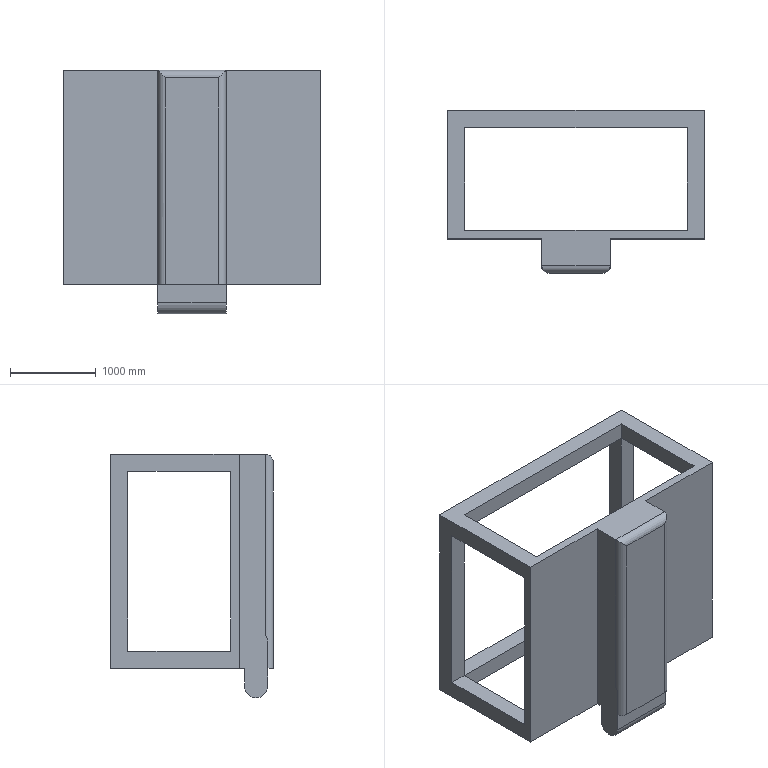Part | SolidWorks | features ICE 6, Extrusion 1, Fillet 1 | 1 solid | 36 faces | box 3000 x 1900 x 2845 mm | volume 2208765977 mm3 | plane 30 | cylinder 6 | commonest cylinder face diameters 180 x3 271.424 x3
STEP:
#1=CARTESIAN_POINT('',(-1300.,300.,10000.));
#2=VERTEX_POINT('',#1);
#3=CARTESIAN_POINT('',(-1300.,1500.,10000.));
#4=VERTEX_POINT('',#3);
#5=CARTESIAN_POINT('',(-1300.,1500.,10000.));
#6=DIRECTION('',(0.,1.,0.));
#7=VECTOR('',#6,1000.);
#8=LINE('',#5,#7);
#9=EDGE_CURVE('',#2,#4,#8,.T.);
#10=ORIENTED_EDGE('',*,*,#9,.F.);
#11=CARTESIAN_POINT('',(1300.,300.,10000.));
#12=VERTEX_POINT('',#11);
#13=CARTESIAN_POINT('',(1300.,300.,10000.));
#14=DIRECTION('',(-1.,0.,0.));
#15=VECTOR('',#14,1000.);
#16=LINE('',#13,#15);
#17=EDGE_CURVE('',#12,#2,#16,.T.);
#18=ORIENTED_EDGE('',*,*,#17,.F.);
#19=CARTESIAN_POINT('',(1300.,1500.,10000.));
#20=VERTEX_POINT('',#19);
#21=CARTESIAN_POINT('',(1300.,1500.,10000.));
#22=DIRECTION('',(0.,-1.,0.));
#23=VECTOR('',#22,1000.);
#24=LINE('',#21,#23);
#25=EDGE_CURVE('',#20,#12,#24,.T.);
#26=ORIENTED_EDGE('',*,*,#25,.F.);
#27=CARTESIAN_POINT('',(1300.,1500.,10000.));
#28=DIRECTION('',(1.,0.,0.));
#29=VECTOR('',#28,1000.);
#30=LINE('',#27,#29);
#31=EDGE_CURVE('',#4,#20,#30,.T.);
#32=ORIENTED_EDGE('',*,*,#31,.F.);
#33=EDGE_LOOP('',(#10,#18,#26,#32));
#34=FACE_BOUND('',#33,.T.);
#35=CARTESIAN_POINT('',(400.,135.712,10000.));
#36=VERTEX_POINT('',#35);
#37=CARTESIAN_POINT('',(400.,200.,10000.));
#38=VERTEX_POINT('',#37);
#39=CARTESIAN_POINT('',(400.,200.,10000.));
#40=DIRECTION('',(0.,1.,0.));
#41=VECTOR('',#40,1000.);
#42=LINE('',#39,#41);
#43=EDGE_CURVE('',#36,#38,#42,.T.);
#44=ORIENTED_EDGE('',*,*,#43,.F.);
#45=CARTESIAN_POINT('',(-400.,135.712,10000.));
#46=VERTEX_POINT('',#45);
#47=CARTESIAN_POINT('',(-1500.,135.712,10000.));
#48=DIRECTION('',(-1.,0.,0.));
#49=VECTOR('',#48,1000.);
#50=LINE('',#47,#49);
#51=EDGE_CURVE('',#36,#46,#50,.T.);
#52=ORIENTED_EDGE('',*,*,#51,.T.);
#53=CARTESIAN_POINT('',(-400.,200.,10000.));
#54=VERTEX_POINT('',#53);
#55=CARTESIAN_POINT('',(-400.,200.,10000.));
#56=DIRECTION('',(0.,-1.,0.));
#57=VECTOR('',#56,1000.);
#58=LINE('',#55,#57);
#59=EDGE_CURVE('',#54,#46,#58,.T.);
#60=ORIENTED_EDGE('',*,*,#59,.F.);
#61=CARTESIAN_POINT('',(-1500.,200.,10000.));
#62=VERTEX_POINT('',#61);
#63=CARTESIAN_POINT('',(-1500.,200.,10000.));
#64=DIRECTION('',(-1.,0.,0.));
#65=VECTOR('',#64,1000.);
#66=LINE('',#63,#65);
#67=EDGE_CURVE('',#54,#62,#66,.T.);
#68=ORIENTED_EDGE('',*,*,#67,.T.);
#69=CARTESIAN_POINT('',(-1500.,1700.,10000.));
#70=VERTEX_POINT('',#69);
#71=CARTESIAN_POINT('',(-1500.,1700.,10000.));
#72=DIRECTION('',(0.,-1.,0.));
#73=VECTOR('',#72,1000.);
#74=LINE('',#71,#73);
#75=EDGE_CURVE('',#70,#62,#74,.T.);
#76=ORIENTED_EDGE('',*,*,#75,.F.);
#77=CARTESIAN_POINT('',(1500.,1700.,10000.));
#78=VERTEX_POINT('',#77);
#79=CARTESIAN_POINT('',(-1500.,1700.,10000.));
#80=DIRECTION('',(-1.,0.,0.));
#81=VECTOR('',#80,1000.);
#82=LINE('',#79,#81);
#83=EDGE_CURVE('',#78,#70,#82,.T.);
#84=ORIENTED_EDGE('',*,*,#83,.F.);
#85=CARTESIAN_POINT('',(1500.,200.,10000.));
#86=VERTEX_POINT('',#85);
#87=CARTESIAN_POINT('',(1500.,1700.,10000.));
#88=DIRECTION('',(0.,-1.,0.));
#89=VECTOR('',#88,1000.);
#90=LINE('',#87,#89);
#91=EDGE_CURVE('',#78,#86,#90,.T.);
#92=ORIENTED_EDGE('',*,*,#91,.T.);
#93=CARTESIAN_POINT('',(-1500.,200.,10000.));
#94=DIRECTION('',(-1.,0.,0.));
#95=VECTOR('',#94,1000.);
#96=LINE('',#93,#95);
#97=EDGE_CURVE('',#86,#38,#96,.T.);
#98=ORIENTED_EDGE('',*,*,#97,.T.);
#99=EDGE_LOOP('',(#44,#52,#60,#68,#76,#84,#92,#98));
#100=FACE_OUTER_BOUND('',#99,.T.);
#101=CARTESIAN_POINT('',(-1500.,1700.,10000.));
#102=DIRECTION('',(0.,0.,1.));
#103=DIRECTION('',(1.,0.,0.));
#104=AXIS2_PLACEMENT_3D('',#101,#102,#103);
#105=PLANE('',#104);
#106=ADVANCED_FACE('',(#34,#100),#105,.F.);
#107=CARTESIAN_POINT('',(400.,-110.,12500.));
#108=VERTEX_POINT('',#107);
#109=CARTESIAN_POINT('',(400.,-110.,10383.617));
#110=VERTEX_POINT('',#109);
#111=CARTESIAN_POINT('',(400.,-110.,12500.));
#112=DIRECTION('',(0.,0.,-1.));
#113=VECTOR('',#112,1000.);
#114=LINE('',#111,#113);
#115=EDGE_CURVE('',#108,#110,#114,.T.);
#116=ORIENTED_EDGE('',*,*,#115,.T.);
#117=CARTESIAN_POINT('',(400.,-135.712,10304.133));
#118=VERTEX_POINT('',#117);
#119=CARTESIAN_POINT('',(400.,0.,10304.133));
#120=DIRECTION('',(1.,0.,0.));
#121=DIRECTION('',(0.,1.,0.));
#122=AXIS2_PLACEMENT_3D('',#119,#120,#121);
#123=CIRCLE('',#122,135.712);
#124=EDGE_CURVE('',#110,#118,#123,.T.);
#125=ORIENTED_EDGE('',*,*,#124,.T.);
#126=CARTESIAN_POINT('',(400.,-135.712,9790.264));
#127=VERTEX_POINT('',#126);
#128=CARTESIAN_POINT('',(400.,-135.712,10304.133));
#129=DIRECTION('',(0.,0.,-1.));
#130=VECTOR('',#129,1000.);
#131=LINE('',#128,#130);
#132=EDGE_CURVE('',#118,#127,#131,.T.);
#133=ORIENTED_EDGE('',*,*,#132,.T.);
#134=CARTESIAN_POINT('',(400.,135.712,9790.264));
#135=VERTEX_POINT('',#134);
#136=CARTESIAN_POINT('',(400.,0.,9790.264));
#137=DIRECTION('',(1.,0.,0.));
#138=DIRECTION('',(0.,1.,0.));
#139=AXIS2_PLACEMENT_3D('',#136,#137,#138);
#140=CIRCLE('',#139,135.712);
#141=EDGE_CURVE('',#127,#135,#140,.T.);
#142=ORIENTED_EDGE('',*,*,#141,.T.);
#143=CARTESIAN_POINT('',(400.,135.712,10304.133));
#144=DIRECTION('',(0.,0.,1.));
#145=VECTOR('',#144,1000.);
#146=LINE('',#143,#145);
#147=EDGE_CURVE('',#135,#36,#146,.T.);
#148=ORIENTED_EDGE('',*,*,#147,.T.);
#149=ORIENTED_EDGE('',*,*,#43,.T.);
#150=CARTESIAN_POINT('',(400.,200.,12500.));
#151=VERTEX_POINT('',#150);
#152=CARTESIAN_POINT('',(400.,200.,12500.));
#153=DIRECTION('',(0.,0.,-1.));
#154=VECTOR('',#153,1000.);
#155=LINE('',#152,#154);
#156=EDGE_CURVE('',#151,#38,#155,.T.);
#157=ORIENTED_EDGE('',*,*,#156,.F.);
#158=CARTESIAN_POINT('',(400.,200.,12500.));
#159=DIRECTION('',(0.,1.,0.));
#160=VECTOR('',#159,1000.);
#161=LINE('',#158,#160);
#162=EDGE_CURVE('',#108,#151,#161,.T.);
#163=ORIENTED_EDGE('',*,*,#162,.F.);
#164=EDGE_LOOP('',(#116,#125,#133,#142,#148,#149,#157,#163));
#165=FACE_OUTER_BOUND('',#164,.T.);
#166=CARTESIAN_POINT('',(400.,200.,12500.));
#167=DIRECTION('',(-1.,0.,0.));
#168=DIRECTION('',(0.,-1.,0.));
#169=AXIS2_PLACEMENT_3D('',#166,#167,#168);
#170=PLANE('',#169);
#171=ADVANCED_FACE('',(#165),#170,.F.);
#172=CARTESIAN_POINT('',(-400.,-135.712,10304.133));
#173=VERTEX_POINT('',#172);
#174=CARTESIAN_POINT('',(-400.,-110.,10383.617));
#175=VERTEX_POINT('',#174);
#176=CARTESIAN_POINT('',(-400.,0.,10304.133));
#177=DIRECTION('',(-1.,0.,0.));
#178=DIRECTION('',(0.,1.,0.));
#179=AXIS2_PLACEMENT_3D('',#176,#177,#178);
#180=CIRCLE('',#179,135.712);
#181=EDGE_CURVE('',#173,#175,#180,.T.);
#182=ORIENTED_EDGE('',*,*,#181,.T.);
#183=CARTESIAN_POINT('',(-400.,-110.,12500.));
#184=VERTEX_POINT('',#183);
#185=CARTESIAN_POINT('',(-400.,-110.,12500.));
#186=DIRECTION('',(0.,0.,1.));
#187=VECTOR('',#186,1000.);
#188=LINE('',#185,#187);
#189=EDGE_CURVE('',#175,#184,#188,.T.);
#190=ORIENTED_EDGE('',*,*,#189,.T.);
#191=CARTESIAN_POINT('',(-400.,200.,12500.));
#192=VERTEX_POINT('',#191);
#193=CARTESIAN_POINT('',(-400.,200.,12500.));
#194=DIRECTION('',(0.,-1.,0.));
#195=VECTOR('',#194,1000.);
#196=LINE('',#193,#195);
#197=EDGE_CURVE('',#192,#184,#196,.T.);
#198=ORIENTED_EDGE('',*,*,#197,.F.);
#199=CARTESIAN_POINT('',(-400.,200.,12500.));
#200=DIRECTION('',(0.,0.,-1.));
#201=VECTOR('',#200,1000.);
#202=LINE('',#199,#201);
#203=EDGE_CURVE('',#192,#54,#202,.T.);
#204=ORIENTED_EDGE('',*,*,#203,.T.);
#205=ORIENTED_EDGE('',*,*,#59,.T.);
#206=CARTESIAN_POINT('',(-400.,135.712,9790.264));
#207=VERTEX_POINT('',#206);
#208=CARTESIAN_POINT('',(-400.,135.712,10304.133));
#209=DIRECTION('',(0.,0.,-1.));
#210=VECTOR('',#209,1000.);
#211=LINE('',#208,#210);
#212=EDGE_CURVE('',#46,#207,#211,.T.);
#213=ORIENTED_EDGE('',*,*,#212,.T.);
#214=CARTESIAN_POINT('',(-400.,-135.712,9790.264));
#215=VERTEX_POINT('',#214);
#216=CARTESIAN_POINT('',(-400.,0.,9790.264));
#217=DIRECTION('',(-1.,0.,0.));
#218=DIRECTION('',(0.,1.,0.));
#219=AXIS2_PLACEMENT_3D('',#216,#217,#218);
#220=CIRCLE('',#219,135.712);
#221=EDGE_CURVE('',#207,#215,#220,.T.);
#222=ORIENTED_EDGE('',*,*,#221,.T.);
#223=CARTESIAN_POINT('',(-400.,-135.712,10304.133));
#224=DIRECTION('',(0.,0.,1.));
#225=VECTOR('',#224,1000.);
#226=LINE('',#223,#225);
#227=EDGE_CURVE('',#215,#173,#226,.T.);
#228=ORIENTED_EDGE('',*,*,#227,.T.);
#229=EDGE_LOOP('',(#182,#190,#198,#204,#205,#213,#222,#228));
#230=FACE_OUTER_BOUND('',#229,.T.);
#231=CARTESIAN_POINT('',(-400.,200.,12500.));
#232=DIRECTION('',(1.,0.,0.));
#233=DIRECTION('',(0.,1.,0.));
#234=AXIS2_PLACEMENT_3D('',#231,#232,#233);
#235=PLANE('',#234);
#236=ADVANCED_FACE('',(#230),#235,.F.);
#237=CARTESIAN_POINT('',(310.,-200.,10000.));
#238=VERTEX_POINT('',#237);
#239=CARTESIAN_POINT('',(-310.,-200.,10000.));
#240=VERTEX_POINT('',#239);
#241=CARTESIAN_POINT('',(-400.,-200.,10000.));
#242=DIRECTION('',(-1.,0.,0.));
#243=VECTOR('',#242,1000.);
#244=LINE('',#241,#243);
#245=EDGE_CURVE('',#238,#240,#244,.T.);
#246=ORIENTED_EDGE('',*,*,#245,.F.);
#247=CARTESIAN_POINT('',(310.,-200.,12410.));
#248=VERTEX_POINT('',#247);
#249=CARTESIAN_POINT('',(310.,-200.,12500.));
#250=DIRECTION('',(0.,0.,1.));
#251=VECTOR('',#250,1000.);
#252=LINE('',#249,#251);
#253=EDGE_CURVE('',#238,#248,#252,.T.);
#254=ORIENTED_EDGE('',*,*,#253,.T.);
#255=CARTESIAN_POINT('',(-310.,-200.,12410.));
#256=VERTEX_POINT('',#255);
#257=CARTESIAN_POINT('',(-400.,-200.,12410.));
#258=DIRECTION('',(-1.,0.,0.));
#259=VECTOR('',#258,1000.);
#260=LINE('',#257,#259);
#261=EDGE_CURVE('',#248,#256,#260,.T.);
#262=ORIENTED_EDGE('',*,*,#261,.T.);
#263=CARTESIAN_POINT('',(-310.,-200.,12500.));
#264=DIRECTION('',(0.,0.,-1.));
#265=VECTOR('',#264,1000.);
#266=LINE('',#263,#265);
#267=EDGE_CURVE('',#256,#240,#266,.T.);
#268=ORIENTED_EDGE('',*,*,#267,.T.);
#269=EDGE_LOOP('',(#246,#254,#262,#268));
#270=FACE_OUTER_BOUND('',#269,.T.);
#271=CARTESIAN_POINT('',(-400.,-200.,12500.));
#272=DIRECTION('',(0.,1.,0.));
#273=DIRECTION('',(0.,0.,1.));
#274=AXIS2_PLACEMENT_3D('',#271,#272,#273);
#275=PLANE('',#274);
#276=ADVANCED_FACE('',(#270),#275,.F.);
#277=CARTESIAN_POINT('',(396.249,-135.712,10304.133));
#278=VERTEX_POINT('',#277);
#279=CARTESIAN_POINT('',(400.,-110.,10383.617));
#280=CARTESIAN_POINT('',(400.,-112.098,10380.714));
#281=CARTESIAN_POINT('',(399.927,-114.065,10377.751));
#282=CARTESIAN_POINT('',(399.685,-117.747,10371.705));
#283=CARTESIAN_POINT('',(399.516,-119.462,10368.624));
#284=CARTESIAN_POINT('',(398.925,-124.237,10359.201));
#285=CARTESIAN_POINT('',(398.422,-126.93,10352.684));
#286=CARTESIAN_POINT('',(397.827,-129.666,10344.227));
#287=CARTESIAN_POINT('',(397.709,-130.183,10342.516));
#288=CARTESIAN_POINT('',(397.482,-131.146,10339.087));
#289=CARTESIAN_POINT('',(397.373,-131.592,10337.368));
#290=CARTESIAN_POINT('',(397.061,-132.826,10332.196));
#291=CARTESIAN_POINT('',(396.877,-133.511,10328.731));
#292=CARTESIAN_POINT('',(396.572,-134.608,10321.765));
#293=CARTESIAN_POINT('',(396.453,-135.021,10318.264));
#294=CARTESIAN_POINT('',(396.291,-135.573,10311.226));
#295=CARTESIAN_POINT('',(396.249,-135.712,10307.689));
#296=CARTESIAN_POINT('',(396.249,-135.712,10304.133));
#297=B_SPLINE_CURVE_WITH_KNOTS('',3,(#279,#280,#281,#282,#283,#284,#285,#286,#287,#288,#289,#290,#291,#292,#293,#294,#295,#296),.UNSPECIFIED.,.F.,.F.,(4,2,2,2,2,2,2,2,4),(0.,0.01058,0.02116,0.04232,0.04761,0.0529,0.06347,0.07405,0.08463),.UNSPECIFIED.);
#298=EDGE_CURVE('',#110,#278,#297,.T.);
#299=ORIENTED_EDGE('',*,*,#298,.F.);
#300=ORIENTED_EDGE('',*,*,#115,.F.);
#301=CARTESIAN_POINT('',(310.,-200.,12410.));
#302=CARTESIAN_POINT('',(362.721,-200.,12462.721));
#303=CARTESIAN_POINT('',(400.,-162.721,12500.));
#304=CARTESIAN_POINT('',(400.,-110.,12500.));
#305=(BOUNDED_CURVE()B_SPLINE_CURVE(3,(#301,#302,#303,#304),.UNSPECIFIED.,.F.,.F.)B_SPLINE_CURVE_WITH_KNOTS((4,4),(1.571,3.142),.UNSPECIFIED.)CURVE()GEOMETRIC_REPRESENTATION_ITEM()RATIONAL_B_SPLINE_CURVE((1.,0.8047,0.8047,1.))REPRESENTATION_ITEM(''));
#306=EDGE_CURVE('',#248,#108,#305,.T.);
#307=ORIENTED_EDGE('',*,*,#306,.F.);
#308=ORIENTED_EDGE('',*,*,#253,.F.);
#309=CARTESIAN_POINT('',(396.249,-135.712,10000.));
#310=VERTEX_POINT('',#309);
#311=CARTESIAN_POINT('',(310.,-110.,10000.));
#312=DIRECTION('',(0.,0.,1.));
#313=DIRECTION('',(-1.,0.,0.));
#314=AXIS2_PLACEMENT_3D('',#311,#312,#313);
#315=CIRCLE('',#314,90.);
#316=EDGE_CURVE('',#238,#310,#315,.T.);
#317=ORIENTED_EDGE('',*,*,#316,.T.);
#318=CARTESIAN_POINT('',(396.249,-135.712,12500.));
#319=DIRECTION('',(0.,0.,-1.));
#320=VECTOR('',#319,1000.);
#321=LINE('',#318,#320);
#322=EDGE_CURVE('',#278,#310,#321,.T.);
#323=ORIENTED_EDGE('',*,*,#322,.F.);
#324=EDGE_LOOP('',(#299,#300,#307,#308,#317,#323));
#325=FACE_OUTER_BOUND('',#324,.T.);
#326=CARTESIAN_POINT('',(310.,-110.,12500.));
#327=DIRECTION('',(0.,0.,-1.));
#328=DIRECTION('',(-1.,0.,0.));
#329=AXIS2_PLACEMENT_3D('',#326,#327,#328);
#330=CYLINDRICAL_SURFACE('',#329,90.);
#331=ADVANCED_FACE('',(#325),#330,.T.);
#332=CARTESIAN_POINT('',(-396.249,-135.712,10304.133));
#333=VERTEX_POINT('',#332);
#334=CARTESIAN_POINT('',(-396.249,-135.712,10304.133));
#335=CARTESIAN_POINT('',(-396.249,-135.712,10305.906));
#336=CARTESIAN_POINT('',(-396.259,-135.677,10307.684));
#337=CARTESIAN_POINT('',(-396.301,-135.537,10311.249));
#338=CARTESIAN_POINT('',(-396.332,-135.432,10313.027));
#339=CARTESIAN_POINT('',(-396.455,-135.014,10318.334));
#340=CARTESIAN_POINT('',(-396.575,-134.598,10321.841));
#341=CARTESIAN_POINT('',(-397.032,-132.949,10332.274));
#342=CARTESIAN_POINT('',(-397.467,-131.317,10339.111));
#343=CARTESIAN_POINT('',(-398.058,-128.604,10347.514));
#344=CARTESIAN_POINT('',(-398.178,-128.027,10349.187));
#345=CARTESIAN_POINT('',(-398.419,-126.806,10352.519));
#346=CARTESIAN_POINT('',(-398.54,-126.159,10354.18));
#347=CARTESIAN_POINT('',(-398.894,-124.13,10359.106));
#348=CARTESIAN_POINT('',(-399.12,-122.654,10362.324));
#349=CARTESIAN_POINT('',(-399.516,-119.459,10368.629));
#350=CARTESIAN_POINT('',(-399.686,-117.74,10371.717));
#351=CARTESIAN_POINT('',(-399.928,-114.056,10377.764));
#352=CARTESIAN_POINT('',(-400.,-112.091,10380.723));
#353=CARTESIAN_POINT('',(-400.,-110.,10383.617));
#354=B_SPLINE_CURVE_WITH_KNOTS('',3,(#334,#335,#336,#337,#338,#339,#340,#341,#342,#343,#344,#345,#346,#347,#348,#349,#350,#351,#352,#353),.UNSPECIFIED.,.F.,.F.,(4,2,2,2,2,2,2,2,2,4),(0.08463,0.08991,0.09518,0.1057,0.1268,0.1321,0.1374,0.1479,0.1585,0.169),.UNSPECIFIED.);
#355=EDGE_CURVE('',#333,#175,#354,.T.);
#356=ORIENTED_EDGE('',*,*,#355,.F.);
#357=CARTESIAN_POINT('',(-396.249,-135.712,10000.));
#358=VERTEX_POINT('',#357);
#359=CARTESIAN_POINT('',(-396.249,-135.712,12500.));
#360=DIRECTION('',(0.,0.,1.));
#361=VECTOR('',#360,1000.);
#362=LINE('',#359,#361);
#363=EDGE_CURVE('',#358,#333,#362,.T.);
#364=ORIENTED_EDGE('',*,*,#363,.F.);
#365=CARTESIAN_POINT('',(-310.,-110.,10000.));
#366=DIRECTION('',(0.,0.,1.));
#367=DIRECTION('',(-1.,0.,0.));
#368=AXIS2_PLACEMENT_3D('',#365,#366,#367);
#369=CIRCLE('',#368,90.);
#370=EDGE_CURVE('',#358,#240,#369,.T.);
#371=ORIENTED_EDGE('',*,*,#370,.T.);
#372=ORIENTED_EDGE('',*,*,#267,.F.);
#373=CARTESIAN_POINT('',(-310.,-200.,12410.));
#374=CARTESIAN_POINT('',(-362.721,-200.,12462.721));
#375=CARTESIAN_POINT('',(-400.,-162.721,12500.));
#376=CARTESIAN_POINT('',(-400.,-110.,12500.));
#377=(BOUNDED_CURVE()B_SPLINE_CURVE(3,(#373,#374,#375,#376),.UNSPECIFIED.,.F.,.F.)B_SPLINE_CURVE_WITH_KNOTS((4,4),(4.712,6.283),.UNSPECIFIED.)CURVE()GEOMETRIC_REPRESENTATION_ITEM()RATIONAL_B_SPLINE_CURVE((1.,0.8047,0.8047,1.))REPRESENTATION_ITEM(''));
#378=EDGE_CURVE('',#256,#184,#377,.T.);
#379=ORIENTED_EDGE('',*,*,#378,.T.);
#380=ORIENTED_EDGE('',*,*,#189,.F.);
#381=EDGE_LOOP('',(#356,#364,#371,#372,#379,#380));
#382=FACE_OUTER_BOUND('',#381,.T.);
#383=CARTESIAN_POINT('',(-310.,-110.,12500.));
#384=DIRECTION('',(0.,0.,-1.));
#385=DIRECTION('',(-1.,0.,0.));
#386=AXIS2_PLACEMENT_3D('',#383,#384,#385);
#387=CYLINDRICAL_SURFACE('',#386,90.);
#388=ADVANCED_FACE('',(#382),#387,.T.);
#389=CARTESIAN_POINT('',(-1500.,1500.,10200.));
#390=VERTEX_POINT('',#389);
#391=CARTESIAN_POINT('',(-1300.,1500.,10200.));
#392=VERTEX_POINT('',#391);
#393=CARTESIAN_POINT('',(-1500.,1500.,10200.));
#394=DIRECTION('',(1.,0.,0.));
#395=VECTOR('',#394,1000.);
#396=LINE('',#393,#395);
#397=EDGE_CURVE('',#390,#392,#396,.T.);
#398=ORIENTED_EDGE('',*,*,#397,.T.);
#399=CARTESIAN_POINT('',(-1300.,1500.,12300.));
#400=VERTEX_POINT('',#399);
#401=CARTESIAN_POINT('',(-1300.,1500.,12300.));
#402=DIRECTION('',(0.,0.,1.));
#403=VECTOR('',#402,1000.);
#404=LINE('',#401,#403);
#405=EDGE_CURVE('',#392,#400,#404,.T.);
#406=ORIENTED_EDGE('',*,*,#405,.T.);
#407=CARTESIAN_POINT('',(-1500.,1500.,12300.));
#408=VERTEX_POINT('',#407);
#409=CARTESIAN_POINT('',(-1500.,1500.,12300.));
#410=DIRECTION('',(1.,0.,0.));
#411=VECTOR('',#410,1000.);
#412=LINE('',#409,#411);
#413=EDGE_CURVE('',#408,#400,#412,.T.);
#414=ORIENTED_EDGE('',*,*,#413,.F.);
#415=CARTESIAN_POINT('',(-1500.,1500.,12300.));
#416=DIRECTION('',(0.,0.,1.));
#417=VECTOR('',#416,1000.);
#418=LINE('',#415,#417);
#419=EDGE_CURVE('',#390,#408,#418,.T.);
#420=ORIENTED_EDGE('',*,*,#419,.F.);
#421=EDGE_LOOP('',(#398,#406,#414,#420));
#422=FACE_OUTER_BOUND('',#421,.T.);
#423=CARTESIAN_POINT('',(-1500.,1500.,12300.));
#424=DIRECTION('',(0.,1.,0.));
#425=DIRECTION('',(0.,0.,1.));
#426=AXIS2_PLACEMENT_3D('',#423,#424,#425);
#427=PLANE('',#426);
#428=ADVANCED_FACE('',(#422),#427,.F.);
#429=CARTESIAN_POINT('',(1300.,1500.,10200.));
#430=VERTEX_POINT('',#429);
#431=CARTESIAN_POINT('',(1300.,1500.,13000.));
#432=DIRECTION('',(0.,0.,-1.));
#433=VECTOR('',#432,1000.);
#434=LINE('',#431,#433);
#435=EDGE_CURVE('',#430,#20,#434,.T.);
#436=ORIENTED_EDGE('',*,*,#435,.F.);
#437=CARTESIAN_POINT('',(-1500.,1500.,10200.));
#438=DIRECTION('',(-1.,0.,0.));
#439=VECTOR('',#438,1000.);
#440=LINE('',#437,#439);
#441=EDGE_CURVE('',#430,#392,#440,.T.);
#442=ORIENTED_EDGE('',*,*,#441,.T.);
#443=CARTESIAN_POINT('',(-1300.,1500.,13000.));
#444=DIRECTION('',(0.,0.,-1.));
#445=VECTOR('',#444,1000.);
#446=LINE('',#443,#445);
#447=EDGE_CURVE('',#392,#4,#446,.T.);
#448=ORIENTED_EDGE('',*,*,#447,.T.);
#449=ORIENTED_EDGE('',*,*,#31,.T.);
#450=EDGE_LOOP('',(#436,#442,#448,#449));
#451=FACE_OUTER_BOUND('',#450,.T.);
#452=CARTESIAN_POINT('',(-1500.,1500.,12300.));
#453=DIRECTION('',(0.,1.,0.));
#454=DIRECTION('',(0.,0.,1.));
#455=AXIS2_PLACEMENT_3D('',#452,#453,#454);
#456=PLANE('',#455);
#457=ADVANCED_FACE('',(#451),#456,.F.);
#458=CARTESIAN_POINT('',(1300.,1500.,12300.));
#459=VERTEX_POINT('',#458);
#460=CARTESIAN_POINT('',(1500.,1500.,12300.));
#461=VERTEX_POINT('',#460);
#462=CARTESIAN_POINT('',(-1500.,1500.,12300.));
#463=DIRECTION('',(1.,0.,0.));
#464=VECTOR('',#463,1000.);
#465=LINE('',#462,#464);
#466=EDGE_CURVE('',#459,#461,#465,.T.);
#467=ORIENTED_EDGE('',*,*,#466,.F.);
#468=CARTESIAN_POINT('',(1300.,1500.,12300.));
#469=DIRECTION('',(0.,0.,-1.));
#470=VECTOR('',#469,1000.);
#471=LINE('',#468,#470);
#472=EDGE_CURVE('',#459,#430,#471,.T.);
#473=ORIENTED_EDGE('',*,*,#472,.T.);
#474=CARTESIAN_POINT('',(1500.,1500.,10200.));
#475=VERTEX_POINT('',#474);
#476=CARTESIAN_POINT('',(-1500.,1500.,10200.));
#477=DIRECTION('',(1.,0.,0.));
#478=VECTOR('',#477,1000.);
#479=LINE('',#476,#478);
#480=EDGE_CURVE('',#430,#475,#479,.T.);
#481=ORIENTED_EDGE('',*,*,#480,.T.);
#482=CARTESIAN_POINT('',(1500.,1500.,12300.));
#483=DIRECTION('',(0.,0.,1.));
#484=VECTOR('',#483,1000.);
#485=LINE('',#482,#484);
#486=EDGE_CURVE('',#475,#461,#485,.T.);
#487=ORIENTED_EDGE('',*,*,#486,.T.);
#488=EDGE_LOOP('',(#467,#473,#481,#487));
#489=FACE_OUTER_BOUND('',#488,.T.);
#490=CARTESIAN_POINT('',(-1500.,1500.,12300.));
#491=DIRECTION('',(0.,1.,0.));
#492=DIRECTION('',(0.,0.,1.));
#493=AXIS2_PLACEMENT_3D('',#490,#491,#492);
#494=PLANE('',#493);
#495=ADVANCED_FACE('',(#489),#494,.F.);
#496=CARTESIAN_POINT('',(1300.,300.,12300.));
#497=VERTEX_POINT('',#496);
#498=CARTESIAN_POINT('',(1500.,300.,12300.));
#499=VERTEX_POINT('',#498);
#500=CARTESIAN_POINT('',(-1500.,300.,12300.));
#501=DIRECTION('',(1.,0.,0.));
#502=VECTOR('',#501,1000.);
#503=LINE('',#500,#502);
#504=EDGE_CURVE('',#497,#499,#503,.T.);
#505=ORIENTED_EDGE('',*,*,#504,.F.);
#506=CARTESIAN_POINT('',(1300.,1500.,12300.));
#507=DIRECTION('',(0.,1.,0.));
#508=VECTOR('',#507,1000.);
#509=LINE('',#506,#508);
#510=EDGE_CURVE('',#497,#459,#509,.T.);
#511=ORIENTED_EDGE('',*,*,#510,.T.);
#512=ORIENTED_EDGE('',*,*,#466,.T.);
#513=CARTESIAN_POINT('',(1500.,1500.,12300.));
#514=DIRECTION('',(0.,-1.,0.));
#515=VECTOR('',#514,1000.);
#516=LINE('',#513,#515);
#517=EDGE_CURVE('',#461,#499,#516,.T.);
#518=ORIENTED_EDGE('',*,*,#517,.T.);
#519=EDGE_LOOP('',(#505,#511,#512,#518));
#520=FACE_OUTER_BOUND('',#519,.T.);
#521=CARTESIAN_POINT('',(-1500.,1500.,12300.));
#522=DIRECTION('',(0.,0.,1.));
#523=DIRECTION('',(1.,0.,0.));
#524=AXIS2_PLACEMENT_3D('',#521,#522,#523);
#525=PLANE('',#524);
#526=ADVANCED_FACE('',(#520),#525,.F.);
#527=ORIENTED_EDGE('',*,*,#480,.F.);
#528=CARTESIAN_POINT('',(1300.,300.,10200.));
#529=VERTEX_POINT('',#528);
#530=CARTESIAN_POINT('',(1300.,1500.,10200.));
#531=DIRECTION('',(0.,-1.,0.));
#532=VECTOR('',#531,1000.);
#533=LINE('',#530,#532);
#534=EDGE_CURVE('',#430,#529,#533,.T.);
#535=ORIENTED_EDGE('',*,*,#534,.T.);
#536=CARTESIAN_POINT('',(1500.,300.,10200.));
#537=VERTEX_POINT('',#536);
#538=CARTESIAN_POINT('',(-1500.,300.,10200.));
#539=DIRECTION('',(1.,0.,0.));
#540=VECTOR('',#539,1000.);
#541=LINE('',#538,#540);
#542=EDGE_CURVE('',#529,#537,#541,.T.);
#543=ORIENTED_EDGE('',*,*,#542,.T.);
#544=CARTESIAN_POINT('',(1500.,1500.,10200.));
#545=DIRECTION('',(0.,1.,0.));
#546=VECTOR('',#545,1000.);
#547=LINE('',#544,#546);
#548=EDGE_CURVE('',#537,#475,#547,.T.);
#549=ORIENTED_EDGE('',*,*,#548,.T.);
#550=EDGE_LOOP('',(#527,#535,#543,#549));
#551=FACE_OUTER_BOUND('',#550,.T.);
#552=CARTESIAN_POINT('',(-1500.,1500.,10200.));
#553=DIRECTION('',(0.,0.,-1.));
#554=DIRECTION('',(-1.,0.,0.));
#555=AXIS2_PLACEMENT_3D('',#552,#553,#554);
#556=PLANE('',#555);
#557=ADVANCED_FACE('',(#551),#556,.F.);
#558=CARTESIAN_POINT('',(1300.,300.,12500.));
#559=VERTEX_POINT('',#558);
#560=CARTESIAN_POINT('',(1300.,1500.,12500.));
#561=VERTEX_POINT('',#560);
#562=CARTESIAN_POINT('',(1300.,0.,12500.));
#563=DIRECTION('',(0.,1.,0.));
#564=VECTOR('',#563,1000.);
#565=LINE('',#562,#564);
#566=EDGE_CURVE('',#559,#561,#565,.T.);
#567=ORIENTED_EDGE('',*,*,#566,.F.);
#568=CARTESIAN_POINT('',(-1300.,300.,12500.));
#569=VERTEX_POINT('',#568);
#570=CARTESIAN_POINT('',(0.,300.,12500.));
#571=DIRECTION('',(1.,0.,0.));
#572=VECTOR('',#571,1000.);
#573=LINE('',#570,#572);
#574=EDGE_CURVE('',#569,#559,#573,.T.);
#575=ORIENTED_EDGE('',*,*,#574,.F.);
#576=CARTESIAN_POINT('',(-1300.,1500.,12500.));
#577=VERTEX_POINT('',#576);
#578=CARTESIAN_POINT('',(-1300.,0.,12500.));
#579=DIRECTION('',(0.,-1.,0.));
#580=VECTOR('',#579,1000.);
#581=LINE('',#578,#580);
#582=EDGE_CURVE('',#577,#569,#581,.T.);
#583=ORIENTED_EDGE('',*,*,#582,.F.);
#584=CARTESIAN_POINT('',(0.,1500.,12500.));
#585=DIRECTION('',(-1.,0.,0.));
#586=VECTOR('',#585,1000.);
#587=LINE('',#584,#586);
#588=EDGE_CURVE('',#561,#577,#587,.T.);
#589=ORIENTED_EDGE('',*,*,#588,.F.);
#590=EDGE_LOOP('',(#567,#575,#583,#589));
#591=FACE_BOUND('',#590,.T.);
#592=ORIENTED_EDGE('',*,*,#197,.T.);
#593=CARTESIAN_POINT('',(400.,-110.,12500.));
#594=DIRECTION('',(1.,0.,0.));
#595=VECTOR('',#594,1000.);
#596=LINE('',#593,#595);
#597=EDGE_CURVE('',#184,#108,#596,.T.);
#598=ORIENTED_EDGE('',*,*,#597,.T.);
#599=ORIENTED_EDGE('',*,*,#162,.T.);
#600=CARTESIAN_POINT('',(1500.,200.,12500.));
#601=VERTEX_POINT('',#600);
#602=CARTESIAN_POINT('',(-1500.,200.,12500.));
#603=DIRECTION('',(1.,0.,0.));
#604=VECTOR('',#603,1000.);
#605=LINE('',#602,#604);
#606=EDGE_CURVE('',#151,#601,#605,.T.);
#607=ORIENTED_EDGE('',*,*,#606,.T.);
#608=CARTESIAN_POINT('',(1500.,1700.,12500.));
#609=VERTEX_POINT('',#608);
#610=CARTESIAN_POINT('',(1500.,1700.,12500.));
#611=DIRECTION('',(0.,-1.,0.));
#612=VECTOR('',#611,1000.);
#613=LINE('',#610,#612);
#614=EDGE_CURVE('',#609,#601,#613,.T.);
#615=ORIENTED_EDGE('',*,*,#614,.F.);
#616=CARTESIAN_POINT('',(-1500.,1700.,12500.));
#617=VERTEX_POINT('',#616);
#618=CARTESIAN_POINT('',(-1500.,1700.,12500.));
#619=DIRECTION('',(1.,0.,0.));
#620=VECTOR('',#619,1000.);
#621=LINE('',#618,#620);
#622=EDGE_CURVE('',#617,#609,#621,.T.);
#623=ORIENTED_EDGE('',*,*,#622,.F.);
#624=CARTESIAN_POINT('',(-1500.,200.,12500.));
#625=VERTEX_POINT('',#624);
#626=CARTESIAN_POINT('',(-1500.,1700.,12500.));
#627=DIRECTION('',(0.,-1.,0.));
#628=VECTOR('',#627,1000.);
#629=LINE('',#626,#628);
#630=EDGE_CURVE('',#617,#625,#629,.T.);
#631=ORIENTED_EDGE('',*,*,#630,.T.);
#632=CARTESIAN_POINT('',(-1500.,200.,12500.));
#633=DIRECTION('',(1.,0.,0.));
#634=VECTOR('',#633,1000.);
#635=LINE('',#632,#634);
#636=EDGE_CURVE('',#625,#192,#635,.T.);
#637=ORIENTED_EDGE('',*,*,#636,.T.);
#638=EDGE_LOOP('',(#592,#598,#599,#607,#615,#623,#631,#637));
#639=FACE_OUTER_BOUND('',#638,.T.);
#640=CARTESIAN_POINT('',(0.,0.,12500.));
#641=DIRECTION('',(0.,0.,1.));
#642=DIRECTION('',(1.,0.,0.));
#643=AXIS2_PLACEMENT_3D('',#640,#641,#642);
#644=PLANE('',#643);
#645=ADVANCED_FACE('',(#591,#639),#644,.T.);
#646=ORIENTED_EDGE('',*,*,#606,.F.);
#647=ORIENTED_EDGE('',*,*,#156,.T.);
#648=ORIENTED_EDGE('',*,*,#97,.F.);
#649=CARTESIAN_POINT('',(1500.,200.,10000.));
#650=DIRECTION('',(0.,0.,-1.));
#651=VECTOR('',#650,1000.);
#652=LINE('',#649,#651);
#653=EDGE_CURVE('',#601,#86,#652,.T.);
#654=ORIENTED_EDGE('',*,*,#653,.F.);
#655=EDGE_LOOP('',(#646,#647,#648,#654));
#656=FACE_OUTER_BOUND('',#655,.T.);
#657=CARTESIAN_POINT('',(0.,200.,0.));
#658=DIRECTION('',(0.,1.,0.));
#659=DIRECTION('',(0.,0.,1.));
#660=AXIS2_PLACEMENT_3D('',#657,#658,#659);
#661=PLANE('',#660);
#662=ADVANCED_FACE('',(#656),#661,.F.);
#663=CARTESIAN_POINT('',(1500.,300.,12300.));
#664=DIRECTION('',(0.,0.,-1.));
#665=VECTOR('',#664,1000.);
#666=LINE('',#663,#665);
#667=EDGE_CURVE('',#499,#537,#666,.T.);
#668=ORIENTED_EDGE('',*,*,#667,.F.);
#669=ORIENTED_EDGE('',*,*,#517,.F.);
#670=ORIENTED_EDGE('',*,*,#486,.F.);
#671=ORIENTED_EDGE('',*,*,#548,.F.);
#672=EDGE_LOOP('',(#668,#669,#670,#671));
#673=FACE_BOUND('',#672,.T.);
#674=ORIENTED_EDGE('',*,*,#653,.T.);
#675=ORIENTED_EDGE('',*,*,#91,.F.);
#676=CARTESIAN_POINT('',(1500.,1700.,10000.));
#677=DIRECTION('',(0.,0.,-1.));
#678=VECTOR('',#677,1000.);
#679=LINE('',#676,#678);
#680=EDGE_CURVE('',#609,#78,#679,.T.);
#681=ORIENTED_EDGE('',*,*,#680,.F.);
#682=ORIENTED_EDGE('',*,*,#614,.T.);
#683=EDGE_LOOP('',(#674,#675,#681,#682));
#684=FACE_OUTER_BOUND('',#683,.T.);
#685=CARTESIAN_POINT('',(1500.,1700.,10000.));
#686=DIRECTION('',(-1.,0.,0.));
#687=DIRECTION('',(0.,0.,1.));
#688=AXIS2_PLACEMENT_3D('',#685,#686,#687);
#689=PLANE('',#688);
#690=ADVANCED_FACE('',(#673,#684),#689,.F.);
#691=ORIENTED_EDGE('',*,*,#370,.F.);
#692=CARTESIAN_POINT('',(-1500.,-135.712,10000.));
#693=DIRECTION('',(1.,0.,0.));
#694=VECTOR('',#693,1000.);
#695=LINE('',#692,#694);
#696=EDGE_CURVE('',#358,#310,#695,.T.);
#697=ORIENTED_EDGE('',*,*,#696,.T.);
#698=ORIENTED_EDGE('',*,*,#316,.F.);
#699=ORIENTED_EDGE('',*,*,#245,.T.);
#700=EDGE_LOOP('',(#691,#697,#698,#699));
#701=FACE_OUTER_BOUND('',#700,.T.);
#702=CARTESIAN_POINT('',(-1500.,1700.,10000.));
#703=DIRECTION('',(0.,0.,1.));
#704=DIRECTION('',(1.,0.,0.));
#705=AXIS2_PLACEMENT_3D('',#702,#703,#704);
#706=PLANE('',#705);
#707=ADVANCED_FACE('',(#701),#706,.F.);
#708=ORIENTED_EDGE('',*,*,#419,.T.);
#709=CARTESIAN_POINT('',(-1500.,300.,12300.));
#710=VERTEX_POINT('',#709);
#711=CARTESIAN_POINT('',(-1500.,1500.,12300.));
#712=DIRECTION('',(0.,-1.,0.));
#713=VECTOR('',#712,1000.);
#714=LINE('',#711,#713);
#715=EDGE_CURVE('',#408,#710,#714,.T.);
#716=ORIENTED_EDGE('',*,*,#715,.T.);
#717=CARTESIAN_POINT('',(-1500.,300.,10200.));
#718=VERTEX_POINT('',#717);
#719=CARTESIAN_POINT('',(-1500.,300.,12300.));
#720=DIRECTION('',(0.,0.,-1.));
#721=VECTOR('',#720,1000.);
#722=LINE('',#719,#721);
#723=EDGE_CURVE('',#710,#718,#722,.T.);
#724=ORIENTED_EDGE('',*,*,#723,.T.);
#725=CARTESIAN_POINT('',(-1500.,1500.,10200.));
#726=DIRECTION('',(0.,1.,0.));
#727=VECTOR('',#726,1000.);
#728=LINE('',#725,#727);
#729=EDGE_CURVE('',#718,#390,#728,.T.);
#730=ORIENTED_EDGE('',*,*,#729,.T.);
#731=EDGE_LOOP('',(#708,#716,#724,#730));
#732=FACE_BOUND('',#731,.T.);
#733=CARTESIAN_POINT('',(-1500.,200.,10000.));
#734=DIRECTION('',(0.,0.,1.));
#735=VECTOR('',#734,1000.);
#736=LINE('',#733,#735);
#737=EDGE_CURVE('',#62,#625,#736,.T.);
#738=ORIENTED_EDGE('',*,*,#737,.T.);
#739=ORIENTED_EDGE('',*,*,#630,.F.);
#740=CARTESIAN_POINT('',(-1500.,1700.,10000.));
#741=DIRECTION('',(0.,0.,1.));
#742=VECTOR('',#741,1000.);
#743=LINE('',#740,#742);
#744=EDGE_CURVE('',#70,#617,#743,.T.);
#745=ORIENTED_EDGE('',*,*,#744,.F.);
#746=ORIENTED_EDGE('',*,*,#75,.T.);
#747=EDGE_LOOP('',(#738,#739,#745,#746));
#748=FACE_OUTER_BOUND('',#747,.T.);
#749=CARTESIAN_POINT('',(-1500.,1700.,10000.));
#750=DIRECTION('',(1.,0.,0.));
#751=DIRECTION('',(0.,0.,-1.));
#752=AXIS2_PLACEMENT_3D('',#749,#750,#751);
#753=PLANE('',#752);
#754=ADVANCED_FACE('',(#732,#748),#753,.F.);
#755=CARTESIAN_POINT('',(-1300.,1700.,10200.));
#756=VERTEX_POINT('',#755);
#757=CARTESIAN_POINT('',(-1300.,1700.,12300.));
#758=VERTEX_POINT('',#757);
#759=CARTESIAN_POINT('',(-1300.,1700.,10200.));
#760=DIRECTION('',(0.,0.,1.));
#761=VECTOR('',#760,1000.);
#762=LINE('',#759,#761);
#763=EDGE_CURVE('',#756,#758,#762,.T.);
#764=ORIENTED_EDGE('',*,*,#763,.F.);
#765=CARTESIAN_POINT('',(1300.,1700.,10200.));
#766=VERTEX_POINT('',#765);
#767=CARTESIAN_POINT('',(-1300.,1700.,10200.));
#768=DIRECTION('',(-1.,0.,0.));
#769=VECTOR('',#768,1000.);
#770=LINE('',#767,#769);
#771=EDGE_CURVE('',#766,#756,#770,.T.);
#772=ORIENTED_EDGE('',*,*,#771,.F.);
#773=CARTESIAN_POINT('',(1300.,1700.,12300.));
#774=VERTEX_POINT('',#773);
#775=CARTESIAN_POINT('',(1300.,1700.,10200.));
#776=DIRECTION('',(0.,0.,-1.));
#777=VECTOR('',#776,1000.);
#778=LINE('',#775,#777);
#779=EDGE_CURVE('',#774,#766,#778,.T.);
#780=ORIENTED_EDGE('',*,*,#779,.F.);
#781=CARTESIAN_POINT('',(-1300.,1700.,12300.));
#782=DIRECTION('',(1.,0.,0.));
#783=VECTOR('',#782,1000.);
#784=LINE('',#781,#783);
#785=EDGE_CURVE('',#758,#774,#784,.T.);
#786=ORIENTED_EDGE('',*,*,#785,.F.);
#787=EDGE_LOOP('',(#764,#772,#780,#786));
#788=FACE_BOUND('',#787,.T.);
#789=ORIENTED_EDGE('',*,*,#680,.T.);
#790=ORIENTED_EDGE('',*,*,#83,.T.);
#791=ORIENTED_EDGE('',*,*,#744,.T.);
#792=ORIENTED_EDGE('',*,*,#622,.T.);
#793=EDGE_LOOP('',(#789,#790,#791,#792));
#794=FACE_OUTER_BOUND('',#793,.T.);
#795=CARTESIAN_POINT('',(0.,1700.,0.));
#796=DIRECTION('',(0.,1.,0.));
#797=DIRECTION('',(0.,0.,1.));
#798=AXIS2_PLACEMENT_3D('',#795,#796,#797);
#799=PLANE('',#798);
#800=ADVANCED_FACE('',(#788,#794),#799,.T.);
#801=ORIENTED_EDGE('',*,*,#203,.F.);
#802=ORIENTED_EDGE('',*,*,#636,.F.);
#803=ORIENTED_EDGE('',*,*,#737,.F.);
#804=ORIENTED_EDGE('',*,*,#67,.F.);
#805=EDGE_LOOP('',(#801,#802,#803,#804));
#806=FACE_OUTER_BOUND('',#805,.T.);
#807=CARTESIAN_POINT('',(0.,200.,0.));
#808=DIRECTION('',(0.,1.,0.));
#809=DIRECTION('',(0.,0.,1.));
#810=AXIS2_PLACEMENT_3D('',#807,#808,#809);
#811=PLANE('',#810);
#812=ADVANCED_FACE('',(#806),#811,.F.);
#813=ORIENTED_EDGE('',*,*,#413,.T.);
#814=CARTESIAN_POINT('',(-1300.,300.,12300.));
#815=VERTEX_POINT('',#814);
#816=CARTESIAN_POINT('',(-1300.,1500.,12300.));
#817=DIRECTION('',(0.,-1.,0.));
#818=VECTOR('',#817,1000.);
#819=LINE('',#816,#818);
#820=EDGE_CURVE('',#400,#815,#819,.T.);
#821=ORIENTED_EDGE('',*,*,#820,.T.);
#822=CARTESIAN_POINT('',(-1500.,300.,12300.));
#823=DIRECTION('',(1.,0.,0.));
#824=VECTOR('',#823,1000.);
#825=LINE('',#822,#824);
#826=EDGE_CURVE('',#710,#815,#825,.T.);
#827=ORIENTED_EDGE('',*,*,#826,.F.);
#828=ORIENTED_EDGE('',*,*,#715,.F.);
#829=EDGE_LOOP('',(#813,#821,#827,#828));
#830=FACE_OUTER_BOUND('',#829,.T.);
#831=CARTESIAN_POINT('',(-1500.,1500.,12300.));
#832=DIRECTION('',(0.,0.,1.));
#833=DIRECTION('',(1.,0.,0.));
#834=AXIS2_PLACEMENT_3D('',#831,#832,#833);
#835=PLANE('',#834);
#836=ADVANCED_FACE('',(#830),#835,.F.);
#837=CARTESIAN_POINT('',(-1300.,1500.,13000.));
#838=DIRECTION('',(0.,0.,-1.));
#839=VECTOR('',#838,1000.);
#840=LINE('',#837,#839);
#841=EDGE_CURVE('',#577,#400,#840,.T.);
#842=ORIENTED_EDGE('',*,*,#841,.T.);
#843=CARTESIAN_POINT('',(-1500.,1500.,12300.));
#844=DIRECTION('',(1.,0.,0.));
#845=VECTOR('',#844,1000.);
#846=LINE('',#843,#845);
#847=EDGE_CURVE('',#400,#459,#846,.T.);
#848=ORIENTED_EDGE('',*,*,#847,.T.);
#849=CARTESIAN_POINT('',(1300.,1500.,13000.));
#850=DIRECTION('',(0.,0.,-1.));
#851=VECTOR('',#850,1000.);
#852=LINE('',#849,#851);
#853=EDGE_CURVE('',#561,#459,#852,.T.);
#854=ORIENTED_EDGE('',*,*,#853,.F.);
#855=ORIENTED_EDGE('',*,*,#588,.T.);
#856=EDGE_LOOP('',(#842,#848,#854,#855));
#857=FACE_OUTER_BOUND('',#856,.T.);
#858=CARTESIAN_POINT('',(-1500.,1500.,12300.));
#859=DIRECTION('',(0.,1.,0.));
#860=DIRECTION('',(0.,0.,1.));
#861=AXIS2_PLACEMENT_3D('',#858,#859,#860);
#862=PLANE('',#861);
#863=ADVANCED_FACE('',(#857),#862,.F.);
#864=CARTESIAN_POINT('',(-1300.,300.,10200.));
#865=VERTEX_POINT('',#864);
#866=CARTESIAN_POINT('',(-1500.,300.,10200.));
#867=DIRECTION('',(1.,0.,0.));
#868=VECTOR('',#867,1000.);
#869=LINE('',#866,#868);
#870=EDGE_CURVE('',#718,#865,#869,.T.);
#871=ORIENTED_EDGE('',*,*,#870,.T.);
#872=CARTESIAN_POINT('',(-1300.,1500.,10200.));
#873=DIRECTION('',(0.,1.,0.));
#874=VECTOR('',#873,1000.);
#875=LINE('',#872,#874);
#876=EDGE_CURVE('',#865,#392,#875,.T.);
#877=ORIENTED_EDGE('',*,*,#876,.T.);
#878=ORIENTED_EDGE('',*,*,#397,.F.);
#879=ORIENTED_EDGE('',*,*,#729,.F.);
#880=EDGE_LOOP('',(#871,#877,#878,#879));
#881=FACE_OUTER_BOUND('',#880,.T.);
#882=CARTESIAN_POINT('',(-1500.,1500.,10200.));
#883=DIRECTION('',(0.,0.,-1.));
#884=DIRECTION('',(-1.,0.,0.));
#885=AXIS2_PLACEMENT_3D('',#882,#883,#884);
#886=PLANE('',#885);
#887=ADVANCED_FACE('',(#881),#886,.F.);
#888=ORIENTED_EDGE('',*,*,#826,.T.);
#889=CARTESIAN_POINT('',(-1300.,300.,13000.));
#890=DIRECTION('',(0.,0.,-1.));
#891=VECTOR('',#890,1000.);
#892=LINE('',#889,#891);
#893=EDGE_CURVE('',#569,#815,#892,.T.);
#894=ORIENTED_EDGE('',*,*,#893,.F.);
#895=ORIENTED_EDGE('',*,*,#574,.T.);
#896=CARTESIAN_POINT('',(1300.,300.,13000.));
#897=DIRECTION('',(0.,0.,-1.));
#898=VECTOR('',#897,1000.);
#899=LINE('',#896,#898);
#900=EDGE_CURVE('',#559,#497,#899,.T.);
#901=ORIENTED_EDGE('',*,*,#900,.T.);
#902=ORIENTED_EDGE('',*,*,#504,.T.);
#903=ORIENTED_EDGE('',*,*,#667,.T.);
#904=ORIENTED_EDGE('',*,*,#542,.F.);
#905=CARTESIAN_POINT('',(1300.,300.,13000.));
#906=DIRECTION('',(0.,0.,-1.));
#907=VECTOR('',#906,1000.);
#908=LINE('',#905,#907);
#909=EDGE_CURVE('',#529,#12,#908,.T.);
#910=ORIENTED_EDGE('',*,*,#909,.T.);
#911=ORIENTED_EDGE('',*,*,#17,.T.);
#912=CARTESIAN_POINT('',(-1300.,300.,13000.));
#913=DIRECTION('',(0.,0.,-1.));
#914=VECTOR('',#913,1000.);
#915=LINE('',#912,#914);
#916=EDGE_CURVE('',#865,#2,#915,.T.);
#917=ORIENTED_EDGE('',*,*,#916,.F.);
#918=ORIENTED_EDGE('',*,*,#870,.F.);
#919=ORIENTED_EDGE('',*,*,#723,.F.);
#920=EDGE_LOOP('',(#888,#894,#895,#901,#902,#903,#904,#910,#911,#917,#918,#919));
#921=FACE_OUTER_BOUND('',#920,.T.);
#922=CARTESIAN_POINT('',(-1500.,300.,12300.));
#923=DIRECTION('',(0.,-1.,0.));
#924=DIRECTION('',(0.,0.,-1.));
#925=AXIS2_PLACEMENT_3D('',#922,#923,#924);
#926=PLANE('',#925);
#927=ADVANCED_FACE('',(#921),#926,.F.);
#928=ORIENTED_EDGE('',*,*,#916,.T.);
#929=ORIENTED_EDGE('',*,*,#9,.T.);
#930=ORIENTED_EDGE('',*,*,#447,.F.);
#931=ORIENTED_EDGE('',*,*,#876,.F.);
#932=EDGE_LOOP('',(#928,#929,#930,#931));
#933=FACE_OUTER_BOUND('',#932,.T.);
#934=CARTESIAN_POINT('',(-1300.,1500.,13000.));
#935=DIRECTION('',(-1.,0.,0.));
#936=DIRECTION('',(0.,-1.,0.));
#937=AXIS2_PLACEMENT_3D('',#934,#935,#936);
#938=PLANE('',#937);
#939=ADVANCED_FACE('',(#933),#938,.F.);
#940=ORIENTED_EDGE('',*,*,#435,.T.);
#941=ORIENTED_EDGE('',*,*,#25,.T.);
#942=ORIENTED_EDGE('',*,*,#909,.F.);
#943=ORIENTED_EDGE('',*,*,#534,.F.);
#944=EDGE_LOOP('',(#940,#941,#942,#943));
#945=FACE_OUTER_BOUND('',#944,.T.);
#946=CARTESIAN_POINT('',(1300.,1500.,13000.));
#947=DIRECTION('',(1.,0.,0.));
#948=DIRECTION('',(0.,1.,0.));
#949=AXIS2_PLACEMENT_3D('',#946,#947,#948);
#950=PLANE('',#949);
#951=ADVANCED_FACE('',(#945),#950,.F.);
#952=ORIENTED_EDGE('',*,*,#566,.T.);
#953=ORIENTED_EDGE('',*,*,#853,.T.);
#954=ORIENTED_EDGE('',*,*,#510,.F.);
#955=ORIENTED_EDGE('',*,*,#900,.F.);
#956=EDGE_LOOP('',(#952,#953,#954,#955));
#957=FACE_OUTER_BOUND('',#956,.T.);
#958=CARTESIAN_POINT('',(1300.,1500.,13000.));
#959=DIRECTION('',(1.,0.,0.));
#960=DIRECTION('',(0.,1.,0.));
#961=AXIS2_PLACEMENT_3D('',#958,#959,#960);
#962=PLANE('',#961);
#963=ADVANCED_FACE('',(#957),#962,.F.);
#964=ORIENTED_EDGE('',*,*,#582,.T.);
#965=ORIENTED_EDGE('',*,*,#893,.T.);
#966=ORIENTED_EDGE('',*,*,#820,.F.);
#967=ORIENTED_EDGE('',*,*,#841,.F.);
#968=EDGE_LOOP('',(#964,#965,#966,#967));
#969=FACE_OUTER_BOUND('',#968,.T.);
#970=CARTESIAN_POINT('',(-1300.,1500.,13000.));
#971=DIRECTION('',(-1.,0.,0.));
#972=DIRECTION('',(0.,-1.,0.));
#973=AXIS2_PLACEMENT_3D('',#970,#971,#972);
#974=PLANE('',#973);
#975=ADVANCED_FACE('',(#969),#974,.F.);
#976=CARTESIAN_POINT('',(1300.,700.,12300.));
#977=DIRECTION('',(0.,1.,0.));
#978=VECTOR('',#977,1000.);
#979=LINE('',#976,#978);
#980=EDGE_CURVE('',#459,#774,#979,.T.);
#981=ORIENTED_EDGE('',*,*,#980,.T.);
#982=ORIENTED_EDGE('',*,*,#779,.T.);
#983=CARTESIAN_POINT('',(1300.,700.,10200.));
#984=DIRECTION('',(0.,1.,0.));
#985=VECTOR('',#984,1000.);
#986=LINE('',#983,#985);
#987=EDGE_CURVE('',#430,#766,#986,.T.);
#988=ORIENTED_EDGE('',*,*,#987,.F.);
#989=ORIENTED_EDGE('',*,*,#472,.F.);
#990=EDGE_LOOP('',(#981,#982,#988,#989));
#991=FACE_OUTER_BOUND('',#990,.T.);
#992=CARTESIAN_POINT('',(1300.,700.,10200.));
#993=DIRECTION('',(1.,0.,0.));
#994=DIRECTION('',(0.,0.,-1.));
#995=AXIS2_PLACEMENT_3D('',#992,#993,#994);
#996=PLANE('',#995);
#997=ADVANCED_FACE('',(#991),#996,.F.);
#998=CARTESIAN_POINT('',(-1300.,700.,10200.));
#999=DIRECTION('',(0.,1.,0.));
#1000=VECTOR('',#999,1000.);
#1001=LINE('',#998,#1000);
#1002=EDGE_CURVE('',#392,#756,#1001,.T.);
#1003=ORIENTED_EDGE('',*,*,#1002,.T.);
#1004=ORIENTED_EDGE('',*,*,#763,.T.);
#1005=CARTESIAN_POINT('',(-1300.,700.,12300.));
#1006=DIRECTION('',(0.,1.,0.));
#1007=VECTOR('',#1006,1000.);
#1008=LINE('',#1005,#1007);
#1009=EDGE_CURVE('',#400,#758,#1008,.T.);
#1010=ORIENTED_EDGE('',*,*,#1009,.F.);
#1011=ORIENTED_EDGE('',*,*,#405,.F.);
#1012=EDGE_LOOP('',(#1003,#1004,#1010,#1011));
#1013=FACE_OUTER_BOUND('',#1012,.T.);
#1014=CARTESIAN_POINT('',(-1300.,700.,10200.));
#1015=DIRECTION('',(-1.,0.,0.));
#1016=DIRECTION('',(0.,0.,1.));
#1017=AXIS2_PLACEMENT_3D('',#1014,#1015,#1016);
#1018=PLANE('',#1017);
#1019=ADVANCED_FACE('',(#1013),#1018,.F.);
#1020=ORIENTED_EDGE('',*,*,#987,.T.);
#1021=ORIENTED_EDGE('',*,*,#771,.T.);
#1022=ORIENTED_EDGE('',*,*,#1002,.F.);
#1023=ORIENTED_EDGE('',*,*,#441,.F.);
#1024=EDGE_LOOP('',(#1020,#1021,#1022,#1023));
#1025=FACE_OUTER_BOUND('',#1024,.T.);
#1026=CARTESIAN_POINT('',(-1300.,700.,10200.));
#1027=DIRECTION('',(0.,0.,-1.));
#1028=DIRECTION('',(-1.,0.,0.));
#1029=AXIS2_PLACEMENT_3D('',#1026,#1027,#1028);
#1030=PLANE('',#1029);
#1031=ADVANCED_FACE('',(#1025),#1030,.F.);
#1032=ORIENTED_EDGE('',*,*,#1009,.T.);
#1033=ORIENTED_EDGE('',*,*,#785,.T.);
#1034=ORIENTED_EDGE('',*,*,#980,.F.);
#1035=ORIENTED_EDGE('',*,*,#847,.F.);
#1036=EDGE_LOOP('',(#1032,#1033,#1034,#1035));
#1037=FACE_OUTER_BOUND('',#1036,.T.);
#1038=CARTESIAN_POINT('',(-1300.,700.,12300.));
#1039=DIRECTION('',(0.,0.,1.));
#1040=DIRECTION('',(1.,0.,0.));
#1041=AXIS2_PLACEMENT_3D('',#1038,#1039,#1040);
#1042=PLANE('',#1041);
#1043=ADVANCED_FACE('',(#1037),#1042,.F.);
#1044=ORIENTED_EDGE('',*,*,#306,.T.);
#1045=ORIENTED_EDGE('',*,*,#597,.F.);
#1046=ORIENTED_EDGE('',*,*,#378,.F.);
#1047=ORIENTED_EDGE('',*,*,#261,.F.);
#1048=EDGE_LOOP('',(#1044,#1045,#1046,#1047));
#1049=FACE_OUTER_BOUND('',#1048,.T.);
#1050=CARTESIAN_POINT('',(0.,-110.,12410.));
#1051=DIRECTION('',(-1.,0.,0.));
#1052=DIRECTION('',(0.,0.,1.));
#1053=AXIS2_PLACEMENT_3D('',#1050,#1051,#1052);
#1054=CYLINDRICAL_SURFACE('',#1053,90.);
#1055=ADVANCED_FACE('',(#1049),#1054,.T.);
#1056=ORIENTED_EDGE('',*,*,#124,.F.);
#1057=ORIENTED_EDGE('',*,*,#298,.T.);
#1058=CARTESIAN_POINT('',(-1230.877,-135.712,10304.133));
#1059=DIRECTION('',(1.,0.,0.));
#1060=VECTOR('',#1059,1000.);
#1061=LINE('',#1058,#1060);
#1062=EDGE_CURVE('',#278,#118,#1061,.T.);
#1063=ORIENTED_EDGE('',*,*,#1062,.T.);
#1064=EDGE_LOOP('',(#1056,#1057,#1063));
#1065=FACE_OUTER_BOUND('',#1064,.T.);
#1066=CARTESIAN_POINT('',(-1230.877,0.,10304.133));
#1067=DIRECTION('',(1.,0.,0.));
#1068=DIRECTION('',(0.,1.,0.));
#1069=AXIS2_PLACEMENT_3D('',#1066,#1067,#1068);
#1070=CYLINDRICAL_SURFACE('',#1069,135.712);
#1071=ADVANCED_FACE('',(#1065),#1070,.T.);
#1072=ORIENTED_EDGE('',*,*,#51,.F.);
#1073=ORIENTED_EDGE('',*,*,#147,.F.);
#1074=CARTESIAN_POINT('',(-1230.877,135.712,9790.264));
#1075=DIRECTION('',(1.,0.,0.));
#1076=VECTOR('',#1075,1000.);
#1077=LINE('',#1074,#1076);
#1078=EDGE_CURVE('',#207,#135,#1077,.T.);
#1079=ORIENTED_EDGE('',*,*,#1078,.F.);
#1080=ORIENTED_EDGE('',*,*,#212,.F.);
#1081=EDGE_LOOP('',(#1072,#1073,#1079,#1080));
#1082=FACE_OUTER_BOUND('',#1081,.T.);
#1083=CARTESIAN_POINT('',(-1230.877,135.712,10304.133));
#1084=DIRECTION('',(0.,1.,0.));
#1085=DIRECTION('',(-1.,0.,0.));
#1086=AXIS2_PLACEMENT_3D('',#1083,#1084,#1085);
#1087=PLANE('',#1086);
#1088=ADVANCED_FACE('',(#1082),#1087,.T.);
#1089=CARTESIAN_POINT('',(-1230.877,-135.712,10304.133));
#1090=DIRECTION('',(1.,0.,0.));
#1091=VECTOR('',#1090,1000.);
#1092=LINE('',#1089,#1091);
#1093=EDGE_CURVE('',#173,#333,#1092,.T.);
#1094=ORIENTED_EDGE('',*,*,#1093,.T.);
#1095=ORIENTED_EDGE('',*,*,#355,.T.);
#1096=ORIENTED_EDGE('',*,*,#181,.F.);
#1097=EDGE_LOOP('',(#1094,#1095,#1096));
#1098=FACE_OUTER_BOUND('',#1097,.T.);
#1099=CARTESIAN_POINT('',(-1230.877,0.,10304.133));
#1100=DIRECTION('',(1.,0.,0.));
#1101=DIRECTION('',(0.,1.,0.));
#1102=AXIS2_PLACEMENT_3D('',#1099,#1100,#1101);
#1103=CYLINDRICAL_SURFACE('',#1102,135.712);
#1104=ADVANCED_FACE('',(#1098),#1103,.T.);
#1105=ORIENTED_EDGE('',*,*,#221,.F.);
#1106=ORIENTED_EDGE('',*,*,#1078,.T.);
#1107=ORIENTED_EDGE('',*,*,#141,.F.);
#1108=CARTESIAN_POINT('',(-1230.877,-135.712,9790.264));
#1109=DIRECTION('',(1.,0.,0.));
#1110=VECTOR('',#1109,1000.);
#1111=LINE('',#1108,#1110);
#1112=EDGE_CURVE('',#215,#127,#1111,.T.);
#1113=ORIENTED_EDGE('',*,*,#1112,.F.);
#1114=EDGE_LOOP('',(#1105,#1106,#1107,#1113));
#1115=FACE_OUTER_BOUND('',#1114,.T.);
#1116=CARTESIAN_POINT('',(-1230.877,0.,9790.264));
#1117=DIRECTION('',(1.,0.,0.));
#1118=DIRECTION('',(0.,1.,0.));
#1119=AXIS2_PLACEMENT_3D('',#1116,#1117,#1118);
#1120=CYLINDRICAL_SURFACE('',#1119,135.712);
#1121=ADVANCED_FACE('',(#1115),#1120,.T.);
#1122=ORIENTED_EDGE('',*,*,#1062,.F.);
#1123=ORIENTED_EDGE('',*,*,#322,.T.);
#1124=ORIENTED_EDGE('',*,*,#696,.F.);
#1125=ORIENTED_EDGE('',*,*,#363,.T.);
#1126=ORIENTED_EDGE('',*,*,#1093,.F.);
#1127=ORIENTED_EDGE('',*,*,#227,.F.);
#1128=ORIENTED_EDGE('',*,*,#1112,.T.);
#1129=ORIENTED_EDGE('',*,*,#132,.F.);
#1130=EDGE_LOOP('',(#1122,#1123,#1124,#1125,#1126,#1127,#1128,#1129));
#1131=FACE_OUTER_BOUND('',#1130,.T.);
#1132=CARTESIAN_POINT('',(-1230.877,-135.712,10304.133));
#1133=DIRECTION('',(0.,-1.,0.));
#1134=DIRECTION('',(1.,0.,0.));
#1135=AXIS2_PLACEMENT_3D('',#1132,#1133,#1134);
#1136=PLANE('',#1135);
#1137=ADVANCED_FACE('',(#1131),#1136,.T.);
#1138=CLOSED_SHELL('',(#106,#171,#236,#276,#331,#388,#428,#457,#495,#526,#557,#645,#662,#690,#707,#754,#800,#812,#836,#863,#887,#927,#939,#951,#963,#975,#997,#1019,#1031,#1043,#1055,#1071,#1088,#1104,#1121,#1137));
#1139=MANIFOLD_SOLID_BREP('',#1138);
#1140=CARTESIAN_POINT('',(0.,0.,0.));
#1141=DIRECTION('',(0.,0.,1.));
#1142=DIRECTION('',(1.,0.,0.));
#1143=AXIS2_PLACEMENT_3D('',#1140,#1141,#1142);
#1144=(LENGTH_UNIT()NAMED_UNIT(*)SI_UNIT(.MILLI.,.METRE.));
#1145=UNCERTAINTY_MEASURE_WITH_UNIT(LENGTH_MEASURE(0.00001),#1144,'','');
#1146=(NAMED_UNIT(*)PLANE_ANGLE_UNIT()SI_UNIT($,.RADIAN.));
#1147=(NAMED_UNIT(*)SI_UNIT($,.STERADIAN.)SOLID_ANGLE_UNIT());
#1148=(GEOMETRIC_REPRESENTATION_CONTEXT(3)GLOBAL_UNCERTAINTY_ASSIGNED_CONTEXT((#1145))GLOBAL_UNIT_ASSIGNED_CONTEXT((#1144,#1146,#1147))REPRESENTATION_CONTEXT('',''));
#1149=ADVANCED_BREP_SHAPE_REPRESENTATION('',(#1139,#1143),#1148);